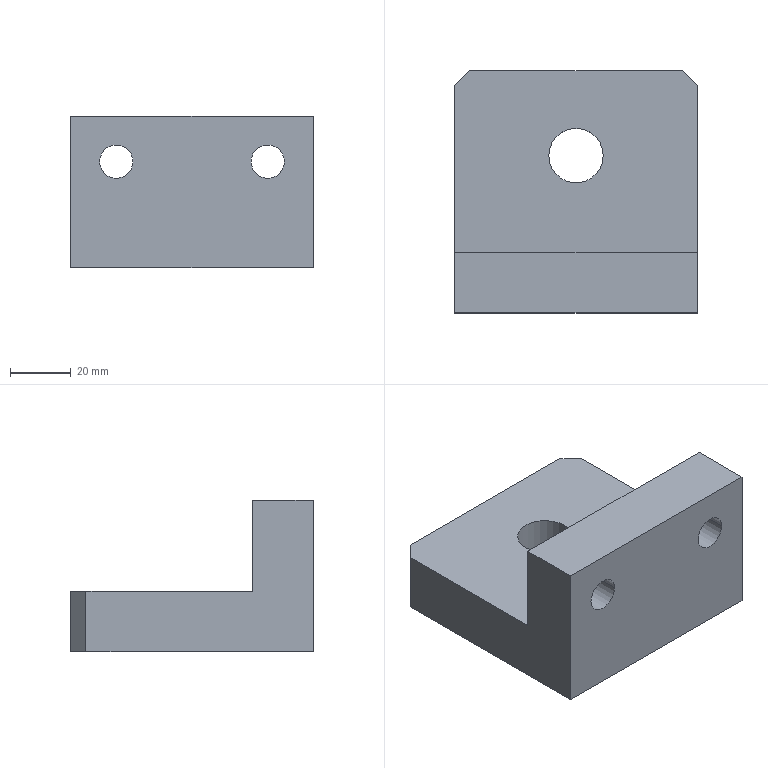Part | STEP file | DCV-000-032-B | 1 solid | 16 faces | box 80 x 80 x 50 mm | volume 166609 mm3 | plane 10 | cylinder 6 | commonest cylinder face diameters 11 x4 18 x2
STEP:
#1=CARTESIAN_POINT('',(0.,0.,0.));
#2=DIRECTION('',(0.,0.,1.));
#3=DIRECTION('',(1.,0.,0.));
#4=AXIS2_PLACEMENT_3D('',#1,#2,#3);
#5=CARTESIAN_POINT('',(30.5,0.,35.));
#6=VERTEX_POINT('',#5);
#7=CARTESIAN_POINT('',(30.5,20.,35.));
#8=VERTEX_POINT('',#7);
#9=CARTESIAN_POINT('',(30.5,-103.693,35.));
#10=DIRECTION('',(0.,1.,0.));
#11=VECTOR('',#10,1.);
#12=LINE('',#9,#11);
#13=CARTESIAN_POINT('',(25.,-103.693,35.));
#14=DIRECTION('',(0.,1.,0.));
#15=DIRECTION('',(1.,0.,0.));
#16=AXIS2_PLACEMENT_3D('',#13,#14,#15);
#17=CYLINDRICAL_SURFACE('',#16,5.5);
#18=CARTESIAN_POINT('',(6.283,0.));
#19=DIRECTION('',(0.,1.));
#20=VECTOR('',#19,1.);
#21=LINE('',#18,#20);
#22=(GEOMETRIC_REPRESENTATION_CONTEXT(2)PARAMETRIC_REPRESENTATION_CONTEXT()REPRESENTATION_CONTEXT('',''));
#23=DEFINITIONAL_REPRESENTATION('',(#21),#22);
#24=PCURVE('',#17,#23);
#25=CARTESIAN_POINT('',(25.,-103.693,35.));
#26=DIRECTION('',(0.,1.,0.));
#27=DIRECTION('',(1.,0.,0.));
#28=AXIS2_PLACEMENT_3D('',#25,#26,#27);
#29=CYLINDRICAL_SURFACE('',#28,5.5);
#30=CARTESIAN_POINT('',(0.,0.));
#31=DIRECTION('',(0.,1.));
#32=VECTOR('',#31,1.);
#33=LINE('',#30,#32);
#34=(GEOMETRIC_REPRESENTATION_CONTEXT(2)PARAMETRIC_REPRESENTATION_CONTEXT()REPRESENTATION_CONTEXT('',''));
#35=DEFINITIONAL_REPRESENTATION('',(#33),#34);
#36=PCURVE('',#29,#35);
#37=SURFACE_CURVE('',#12,(#24,#36),.PCURVE_S1.);
#38=EDGE_CURVE('',#6,#8,#37,.T.);
#39=ORIENTED_EDGE('',*,*,#38,.T.);
#40=CARTESIAN_POINT('',(19.5,20.,35.));
#41=VERTEX_POINT('',#40);
#42=CARTESIAN_POINT('',(25.,20.,35.));
#43=DIRECTION('',(0.,-1.,0.));
#44=DIRECTION('',(1.,0.,0.));
#45=AXIS2_PLACEMENT_3D('',#42,#43,#44);
#46=CIRCLE('',#45,5.5);
#47=CARTESIAN_POINT('',(6.283,123.693));
#48=DIRECTION('',(-1.,0.));
#49=VECTOR('',#48,1.);
#50=LINE('',#47,#49);
#51=(GEOMETRIC_REPRESENTATION_CONTEXT(2)PARAMETRIC_REPRESENTATION_CONTEXT()REPRESENTATION_CONTEXT('',''));
#52=DEFINITIONAL_REPRESENTATION('',(#50),#51);
#53=PCURVE('',#17,#52);
#54=CARTESIAN_POINT('',(40.,20.,20.));
#55=DIRECTION('',(0.,1.,0.));
#56=DIRECTION('',(1.,0.,0.));
#57=AXIS2_PLACEMENT_3D('',#54,#55,#56);
#58=PLANE('',#57);
#59=CARTESIAN_POINT('',(-9.5,-15.));
#60=CARTESIAN_POINT('',(-9.5,-24.526));
#61=CARTESIAN_POINT('',(-17.75,-19.763));
#62=CARTESIAN_POINT('',(-26.,-15.));
#63=CARTESIAN_POINT('',(-17.75,-10.237));
#64=CARTESIAN_POINT('',(-9.5,-5.474));
#65=CARTESIAN_POINT('',(-9.5,-15.));
#66=(BOUNDED_CURVE()B_SPLINE_CURVE(2,(#59,#60,#61,#62,#63,#64,#65),.UNSPECIFIED.,.T.,.F.)B_SPLINE_CURVE_WITH_KNOTS((1,2,2,2,2,1),(-2.094,0.,2.094,4.189,6.283,8.378),.UNSPECIFIED.)CURVE()GEOMETRIC_REPRESENTATION_ITEM()RATIONAL_B_SPLINE_CURVE((1.,0.5,1.,0.5,1.,0.5,1.))REPRESENTATION_ITEM(''));
#67=(GEOMETRIC_REPRESENTATION_CONTEXT(2)PARAMETRIC_REPRESENTATION_CONTEXT()REPRESENTATION_CONTEXT('',''));
#68=DEFINITIONAL_REPRESENTATION('',(#66),#67);
#69=PCURVE('',#58,#68);
#70=SURFACE_CURVE('',#46,(#53,#69),.PCURVE_S1.);
#71=EDGE_CURVE('',#8,#41,#70,.T.);
#72=ORIENTED_EDGE('',*,*,#71,.T.);
#73=CARTESIAN_POINT('',(19.5,0.,35.));
#74=VERTEX_POINT('',#73);
#75=CARTESIAN_POINT('',(19.5,-103.693,35.));
#76=DIRECTION('',(0.,1.,0.));
#77=VECTOR('',#76,1.);
#78=LINE('',#75,#77);
#79=CARTESIAN_POINT('',(3.142,0.));
#80=DIRECTION('',(0.,1.));
#81=VECTOR('',#80,1.);
#82=LINE('',#79,#81);
#83=(GEOMETRIC_REPRESENTATION_CONTEXT(2)PARAMETRIC_REPRESENTATION_CONTEXT()REPRESENTATION_CONTEXT('',''));
#84=DEFINITIONAL_REPRESENTATION('',(#82),#83);
#85=PCURVE('',#17,#84);
#86=CARTESIAN_POINT('',(3.142,0.));
#87=DIRECTION('',(0.,1.));
#88=VECTOR('',#87,1.);
#89=LINE('',#86,#88);
#90=(GEOMETRIC_REPRESENTATION_CONTEXT(2)PARAMETRIC_REPRESENTATION_CONTEXT()REPRESENTATION_CONTEXT('',''));
#91=DEFINITIONAL_REPRESENTATION('',(#89),#90);
#92=PCURVE('',#29,#91);
#93=SURFACE_CURVE('',#78,(#85,#92),.PCURVE_S1.);
#94=EDGE_CURVE('',#74,#41,#93,.T.);
#95=ORIENTED_EDGE('',*,*,#94,.F.);
#96=CARTESIAN_POINT('',(25.,0.,35.));
#97=DIRECTION('',(0.,1.,0.));
#98=DIRECTION('',(1.,0.,0.));
#99=AXIS2_PLACEMENT_3D('',#96,#97,#98);
#100=CIRCLE('',#99,5.5);
#101=CARTESIAN_POINT('',(0.,103.693));
#102=DIRECTION('',(1.,0.));
#103=VECTOR('',#102,1.);
#104=LINE('',#101,#103);
#105=(GEOMETRIC_REPRESENTATION_CONTEXT(2)PARAMETRIC_REPRESENTATION_CONTEXT()REPRESENTATION_CONTEXT('',''));
#106=DEFINITIONAL_REPRESENTATION('',(#104),#105);
#107=PCURVE('',#17,#106);
#108=CARTESIAN_POINT('',(-40.,0.,0.));
#109=DIRECTION('',(0.,-1.,0.));
#110=DIRECTION('',(0.,0.,-1.));
#111=AXIS2_PLACEMENT_3D('',#108,#109,#110);
#112=PLANE('',#111);
#113=CARTESIAN_POINT('',(-35.,70.5));
#114=CARTESIAN_POINT('',(-25.474,70.5));
#115=CARTESIAN_POINT('',(-30.237,62.25));
#116=CARTESIAN_POINT('',(-35.,54.));
#117=CARTESIAN_POINT('',(-39.763,62.25));
#118=CARTESIAN_POINT('',(-44.526,70.5));
#119=CARTESIAN_POINT('',(-35.,70.5));
#120=(BOUNDED_CURVE()B_SPLINE_CURVE(2,(#113,#114,#115,#116,#117,#118,#119),.UNSPECIFIED.,.T.,.F.)B_SPLINE_CURVE_WITH_KNOTS((1,2,2,2,2,1),(-2.094,0.,2.094,4.189,6.283,8.378),.UNSPECIFIED.)CURVE()GEOMETRIC_REPRESENTATION_ITEM()RATIONAL_B_SPLINE_CURVE((1.,0.5,1.,0.5,1.,0.5,1.))REPRESENTATION_ITEM(''));
#121=(GEOMETRIC_REPRESENTATION_CONTEXT(2)PARAMETRIC_REPRESENTATION_CONTEXT()REPRESENTATION_CONTEXT('',''));
#122=DEFINITIONAL_REPRESENTATION('',(#120),#121);
#123=PCURVE('',#112,#122);
#124=SURFACE_CURVE('',#100,(#107,#123),.PCURVE_S1.);
#125=EDGE_CURVE('',#74,#6,#124,.T.);
#126=ORIENTED_EDGE('',*,*,#125,.T.);
#127=EDGE_LOOP('',(#39,#72,#95,#126));
#128=FACE_BOUND('',#127,.F.);
#129=ADVANCED_FACE('',(#128),#17,.F.);
#130=CARTESIAN_POINT('',(-19.5,0.,35.));
#131=VERTEX_POINT('',#130);
#132=CARTESIAN_POINT('',(-19.5,20.,35.));
#133=VERTEX_POINT('',#132);
#134=CARTESIAN_POINT('',(-19.5,-103.693,35.));
#135=DIRECTION('',(0.,1.,0.));
#136=VECTOR('',#135,1.);
#137=LINE('',#134,#136);
#138=CARTESIAN_POINT('',(-25.,-103.693,35.));
#139=DIRECTION('',(0.,1.,0.));
#140=DIRECTION('',(1.,0.,0.));
#141=AXIS2_PLACEMENT_3D('',#138,#139,#140);
#142=CYLINDRICAL_SURFACE('',#141,5.5);
#143=CARTESIAN_POINT('',(6.283,0.));
#144=DIRECTION('',(0.,1.));
#145=VECTOR('',#144,1.);
#146=LINE('',#143,#145);
#147=(GEOMETRIC_REPRESENTATION_CONTEXT(2)PARAMETRIC_REPRESENTATION_CONTEXT()REPRESENTATION_CONTEXT('',''));
#148=DEFINITIONAL_REPRESENTATION('',(#146),#147);
#149=PCURVE('',#142,#148);
#150=CARTESIAN_POINT('',(-25.,-103.693,35.));
#151=DIRECTION('',(0.,1.,0.));
#152=DIRECTION('',(1.,0.,0.));
#153=AXIS2_PLACEMENT_3D('',#150,#151,#152);
#154=CYLINDRICAL_SURFACE('',#153,5.5);
#155=CARTESIAN_POINT('',(0.,0.));
#156=DIRECTION('',(0.,1.));
#157=VECTOR('',#156,1.);
#158=LINE('',#155,#157);
#159=(GEOMETRIC_REPRESENTATION_CONTEXT(2)PARAMETRIC_REPRESENTATION_CONTEXT()REPRESENTATION_CONTEXT('',''));
#160=DEFINITIONAL_REPRESENTATION('',(#158),#159);
#161=PCURVE('',#154,#160);
#162=SURFACE_CURVE('',#137,(#149,#161),.PCURVE_S1.);
#163=EDGE_CURVE('',#131,#133,#162,.T.);
#164=ORIENTED_EDGE('',*,*,#163,.T.);
#165=CARTESIAN_POINT('',(-30.5,20.,35.));
#166=VERTEX_POINT('',#165);
#167=CARTESIAN_POINT('',(-25.,20.,35.));
#168=DIRECTION('',(0.,-1.,0.));
#169=DIRECTION('',(1.,0.,0.));
#170=AXIS2_PLACEMENT_3D('',#167,#168,#169);
#171=CIRCLE('',#170,5.5);
#172=CARTESIAN_POINT('',(6.283,123.693));
#173=DIRECTION('',(-1.,0.));
#174=VECTOR('',#173,1.);
#175=LINE('',#172,#174);
#176=(GEOMETRIC_REPRESENTATION_CONTEXT(2)PARAMETRIC_REPRESENTATION_CONTEXT()REPRESENTATION_CONTEXT('',''));
#177=DEFINITIONAL_REPRESENTATION('',(#175),#176);
#178=PCURVE('',#142,#177);
#179=CARTESIAN_POINT('',(-59.5,-15.));
#180=CARTESIAN_POINT('',(-59.5,-24.526));
#181=CARTESIAN_POINT('',(-67.75,-19.763));
#182=CARTESIAN_POINT('',(-76.,-15.));
#183=CARTESIAN_POINT('',(-67.75,-10.237));
#184=CARTESIAN_POINT('',(-59.5,-5.474));
#185=CARTESIAN_POINT('',(-59.5,-15.));
#186=(BOUNDED_CURVE()B_SPLINE_CURVE(2,(#179,#180,#181,#182,#183,#184,#185),.UNSPECIFIED.,.T.,.F.)B_SPLINE_CURVE_WITH_KNOTS((1,2,2,2,2,1),(-2.094,0.,2.094,4.189,6.283,8.378),.UNSPECIFIED.)CURVE()GEOMETRIC_REPRESENTATION_ITEM()RATIONAL_B_SPLINE_CURVE((1.,0.5,1.,0.5,1.,0.5,1.))REPRESENTATION_ITEM(''));
#187=(GEOMETRIC_REPRESENTATION_CONTEXT(2)PARAMETRIC_REPRESENTATION_CONTEXT()REPRESENTATION_CONTEXT('',''));
#188=DEFINITIONAL_REPRESENTATION('',(#186),#187);
#189=PCURVE('',#58,#188);
#190=SURFACE_CURVE('',#171,(#178,#189),.PCURVE_S1.);
#191=EDGE_CURVE('',#133,#166,#190,.T.);
#192=ORIENTED_EDGE('',*,*,#191,.T.);
#193=CARTESIAN_POINT('',(-30.5,0.,35.));
#194=VERTEX_POINT('',#193);
#195=CARTESIAN_POINT('',(-30.5,-103.693,35.));
#196=DIRECTION('',(0.,1.,0.));
#197=VECTOR('',#196,1.);
#198=LINE('',#195,#197);
#199=CARTESIAN_POINT('',(3.142,0.));
#200=DIRECTION('',(0.,1.));
#201=VECTOR('',#200,1.);
#202=LINE('',#199,#201);
#203=(GEOMETRIC_REPRESENTATION_CONTEXT(2)PARAMETRIC_REPRESENTATION_CONTEXT()REPRESENTATION_CONTEXT('',''));
#204=DEFINITIONAL_REPRESENTATION('',(#202),#203);
#205=PCURVE('',#142,#204);
#206=CARTESIAN_POINT('',(3.142,0.));
#207=DIRECTION('',(0.,1.));
#208=VECTOR('',#207,1.);
#209=LINE('',#206,#208);
#210=(GEOMETRIC_REPRESENTATION_CONTEXT(2)PARAMETRIC_REPRESENTATION_CONTEXT()REPRESENTATION_CONTEXT('',''));
#211=DEFINITIONAL_REPRESENTATION('',(#209),#210);
#212=PCURVE('',#154,#211);
#213=SURFACE_CURVE('',#198,(#205,#212),.PCURVE_S1.);
#214=EDGE_CURVE('',#194,#166,#213,.T.);
#215=ORIENTED_EDGE('',*,*,#214,.F.);
#216=CARTESIAN_POINT('',(-25.,0.,35.));
#217=DIRECTION('',(0.,1.,0.));
#218=DIRECTION('',(1.,0.,0.));
#219=AXIS2_PLACEMENT_3D('',#216,#217,#218);
#220=CIRCLE('',#219,5.5);
#221=CARTESIAN_POINT('',(0.,103.693));
#222=DIRECTION('',(1.,0.));
#223=VECTOR('',#222,1.);
#224=LINE('',#221,#223);
#225=(GEOMETRIC_REPRESENTATION_CONTEXT(2)PARAMETRIC_REPRESENTATION_CONTEXT()REPRESENTATION_CONTEXT('',''));
#226=DEFINITIONAL_REPRESENTATION('',(#224),#225);
#227=PCURVE('',#142,#226);
#228=CARTESIAN_POINT('',(-35.,20.5));
#229=CARTESIAN_POINT('',(-25.474,20.5));
#230=CARTESIAN_POINT('',(-30.237,12.25));
#231=CARTESIAN_POINT('',(-35.,4.));
#232=CARTESIAN_POINT('',(-39.763,12.25));
#233=CARTESIAN_POINT('',(-44.526,20.5));
#234=CARTESIAN_POINT('',(-35.,20.5));
#235=(BOUNDED_CURVE()B_SPLINE_CURVE(2,(#228,#229,#230,#231,#232,#233,#234),.UNSPECIFIED.,.T.,.F.)B_SPLINE_CURVE_WITH_KNOTS((1,2,2,2,2,1),(-2.094,0.,2.094,4.189,6.283,8.378),.UNSPECIFIED.)CURVE()GEOMETRIC_REPRESENTATION_ITEM()RATIONAL_B_SPLINE_CURVE((1.,0.5,1.,0.5,1.,0.5,1.))REPRESENTATION_ITEM(''));
#236=(GEOMETRIC_REPRESENTATION_CONTEXT(2)PARAMETRIC_REPRESENTATION_CONTEXT()REPRESENTATION_CONTEXT('',''));
#237=DEFINITIONAL_REPRESENTATION('',(#235),#236);
#238=PCURVE('',#112,#237);
#239=SURFACE_CURVE('',#220,(#227,#238),.PCURVE_S1.);
#240=EDGE_CURVE('',#194,#131,#239,.T.);
#241=ORIENTED_EDGE('',*,*,#240,.T.);
#242=EDGE_LOOP('',(#164,#192,#215,#241));
#243=FACE_BOUND('',#242,.F.);
#244=ADVANCED_FACE('',(#243),#142,.F.);
#245=CARTESIAN_POINT('',(9.,52.,0.));
#246=VERTEX_POINT('',#245);
#247=CARTESIAN_POINT('',(9.,52.,20.));
#248=VERTEX_POINT('',#247);
#249=CARTESIAN_POINT('',(9.,52.,-94.891));
#250=DIRECTION('',(0.,0.,1.));
#251=VECTOR('',#250,1.);
#252=LINE('',#249,#251);
#253=CARTESIAN_POINT('',(0.,52.,-94.891));
#254=DIRECTION('',(0.,0.,1.));
#255=DIRECTION('',(1.,0.,0.));
#256=AXIS2_PLACEMENT_3D('',#253,#254,#255);
#257=CYLINDRICAL_SURFACE('',#256,9.);
#258=CARTESIAN_POINT('',(6.283,0.));
#259=DIRECTION('',(0.,1.));
#260=VECTOR('',#259,1.);
#261=LINE('',#258,#260);
#262=(GEOMETRIC_REPRESENTATION_CONTEXT(2)PARAMETRIC_REPRESENTATION_CONTEXT()REPRESENTATION_CONTEXT('',''));
#263=DEFINITIONAL_REPRESENTATION('',(#261),#262);
#264=PCURVE('',#257,#263);
#265=CARTESIAN_POINT('',(0.,52.,-94.891));
#266=DIRECTION('',(0.,0.,1.));
#267=DIRECTION('',(1.,0.,0.));
#268=AXIS2_PLACEMENT_3D('',#265,#266,#267);
#269=CYLINDRICAL_SURFACE('',#268,9.);
#270=CARTESIAN_POINT('',(0.,0.));
#271=DIRECTION('',(0.,1.));
#272=VECTOR('',#271,1.);
#273=LINE('',#270,#272);
#274=(GEOMETRIC_REPRESENTATION_CONTEXT(2)PARAMETRIC_REPRESENTATION_CONTEXT()REPRESENTATION_CONTEXT('',''));
#275=DEFINITIONAL_REPRESENTATION('',(#273),#274);
#276=PCURVE('',#269,#275);
#277=SURFACE_CURVE('',#252,(#264,#276),.PCURVE_S1.);
#278=EDGE_CURVE('',#246,#248,#277,.T.);
#279=ORIENTED_EDGE('',*,*,#278,.T.);
#280=CARTESIAN_POINT('',(-9.,52.,20.));
#281=VERTEX_POINT('',#280);
#282=CARTESIAN_POINT('',(0.,52.,20.));
#283=DIRECTION('',(0.,0.,-1.));
#284=DIRECTION('',(1.,0.,0.));
#285=AXIS2_PLACEMENT_3D('',#282,#283,#284);
#286=CIRCLE('',#285,9.);
#287=CARTESIAN_POINT('',(6.283,114.891));
#288=DIRECTION('',(-1.,0.));
#289=VECTOR('',#288,1.);
#290=LINE('',#287,#289);
#291=(GEOMETRIC_REPRESENTATION_CONTEXT(2)PARAMETRIC_REPRESENTATION_CONTEXT()REPRESENTATION_CONTEXT('',''));
#292=DEFINITIONAL_REPRESENTATION('',(#290),#291);
#293=PCURVE('',#257,#292);
#294=CARTESIAN_POINT('',(0.,40.,20.));
#295=DIRECTION('',(0.,0.,1.));
#296=DIRECTION('',(1.,0.,0.));
#297=AXIS2_PLACEMENT_3D('',#294,#295,#296);
#298=PLANE('',#297);
#299=CARTESIAN_POINT('',(9.,12.));
#300=CARTESIAN_POINT('',(9.,-3.588));
#301=CARTESIAN_POINT('',(-4.5,4.206));
#302=CARTESIAN_POINT('',(-18.,12.));
#303=CARTESIAN_POINT('',(-4.5,19.794));
#304=CARTESIAN_POINT('',(9.,27.588));
#305=CARTESIAN_POINT('',(9.,12.));
#306=(BOUNDED_CURVE()B_SPLINE_CURVE(2,(#299,#300,#301,#302,#303,#304,#305),.UNSPECIFIED.,.T.,.F.)B_SPLINE_CURVE_WITH_KNOTS((1,2,2,2,2,1),(-2.094,0.,2.094,4.189,6.283,8.378),.UNSPECIFIED.)CURVE()GEOMETRIC_REPRESENTATION_ITEM()RATIONAL_B_SPLINE_CURVE((1.,0.5,1.,0.5,1.,0.5,1.))REPRESENTATION_ITEM(''));
#307=(GEOMETRIC_REPRESENTATION_CONTEXT(2)PARAMETRIC_REPRESENTATION_CONTEXT()REPRESENTATION_CONTEXT('',''));
#308=DEFINITIONAL_REPRESENTATION('',(#306),#307);
#309=PCURVE('',#298,#308);
#310=SURFACE_CURVE('',#286,(#293,#309),.PCURVE_S1.);
#311=EDGE_CURVE('',#248,#281,#310,.T.);
#312=ORIENTED_EDGE('',*,*,#311,.T.);
#313=CARTESIAN_POINT('',(-9.,52.,0.));
#314=VERTEX_POINT('',#313);
#315=CARTESIAN_POINT('',(-9.,52.,-94.891));
#316=DIRECTION('',(0.,0.,1.));
#317=VECTOR('',#316,1.);
#318=LINE('',#315,#317);
#319=CARTESIAN_POINT('',(3.142,0.));
#320=DIRECTION('',(0.,1.));
#321=VECTOR('',#320,1.);
#322=LINE('',#319,#321);
#323=(GEOMETRIC_REPRESENTATION_CONTEXT(2)PARAMETRIC_REPRESENTATION_CONTEXT()REPRESENTATION_CONTEXT('',''));
#324=DEFINITIONAL_REPRESENTATION('',(#322),#323);
#325=PCURVE('',#257,#324);
#326=CARTESIAN_POINT('',(3.142,0.));
#327=DIRECTION('',(0.,1.));
#328=VECTOR('',#327,1.);
#329=LINE('',#326,#328);
#330=(GEOMETRIC_REPRESENTATION_CONTEXT(2)PARAMETRIC_REPRESENTATION_CONTEXT()REPRESENTATION_CONTEXT('',''));
#331=DEFINITIONAL_REPRESENTATION('',(#329),#330);
#332=PCURVE('',#269,#331);
#333=SURFACE_CURVE('',#318,(#325,#332),.PCURVE_S1.);
#334=EDGE_CURVE('',#314,#281,#333,.T.);
#335=ORIENTED_EDGE('',*,*,#334,.F.);
#336=CARTESIAN_POINT('',(0.,52.,0.));
#337=DIRECTION('',(0.,0.,1.));
#338=DIRECTION('',(1.,0.,0.));
#339=AXIS2_PLACEMENT_3D('',#336,#337,#338);
#340=CIRCLE('',#339,9.);
#341=CARTESIAN_POINT('',(0.,94.891));
#342=DIRECTION('',(1.,0.));
#343=VECTOR('',#342,1.);
#344=LINE('',#341,#343);
#345=(GEOMETRIC_REPRESENTATION_CONTEXT(2)PARAMETRIC_REPRESENTATION_CONTEXT()REPRESENTATION_CONTEXT('',''));
#346=DEFINITIONAL_REPRESENTATION('',(#344),#345);
#347=PCURVE('',#257,#346);
#348=CARTESIAN_POINT('',(0.,40.,0.));
#349=DIRECTION('',(0.,0.,1.));
#350=DIRECTION('',(1.,0.,0.));
#351=AXIS2_PLACEMENT_3D('',#348,#349,#350);
#352=PLANE('',#351);
#353=CARTESIAN_POINT('',(0.,12.));
#354=DIRECTION('',(1.,0.));
#355=AXIS2_PLACEMENT_2D('',#353,#354);
#356=CIRCLE('',#355,9.);
#357=(GEOMETRIC_REPRESENTATION_CONTEXT(2)PARAMETRIC_REPRESENTATION_CONTEXT()REPRESENTATION_CONTEXT('',''));
#358=DEFINITIONAL_REPRESENTATION('',(#356),#357);
#359=PCURVE('',#352,#358);
#360=SURFACE_CURVE('',#340,(#347,#359),.PCURVE_S1.);
#361=EDGE_CURVE('',#314,#246,#360,.T.);
#362=ORIENTED_EDGE('',*,*,#361,.T.);
#363=EDGE_LOOP('',(#279,#312,#335,#362));
#364=FACE_BOUND('',#363,.F.);
#365=ADVANCED_FACE('',(#364),#257,.F.);
#366=ORIENTED_EDGE('',*,*,#311,.T.);
#367=CARTESIAN_POINT('',(0.,52.,20.));
#368=DIRECTION('',(0.,0.,-1.));
#369=DIRECTION('',(1.,0.,0.));
#370=AXIS2_PLACEMENT_3D('',#367,#368,#369);
#371=CIRCLE('',#370,9.);
#372=CARTESIAN_POINT('',(9.,12.));
#373=CARTESIAN_POINT('',(9.,-3.588));
#374=CARTESIAN_POINT('',(-4.5,4.206));
#375=CARTESIAN_POINT('',(-18.,12.));
#376=CARTESIAN_POINT('',(-4.5,19.794));
#377=CARTESIAN_POINT('',(9.,27.588));
#378=CARTESIAN_POINT('',(9.,12.));
#379=(BOUNDED_CURVE()B_SPLINE_CURVE(2,(#372,#373,#374,#375,#376,#377,#378),.UNSPECIFIED.,.T.,.F.)B_SPLINE_CURVE_WITH_KNOTS((1,2,2,2,2,1),(-2.094,0.,2.094,4.189,6.283,8.378),.UNSPECIFIED.)CURVE()GEOMETRIC_REPRESENTATION_ITEM()RATIONAL_B_SPLINE_CURVE((1.,0.5,1.,0.5,1.,0.5,1.))REPRESENTATION_ITEM(''));
#380=(GEOMETRIC_REPRESENTATION_CONTEXT(2)PARAMETRIC_REPRESENTATION_CONTEXT()REPRESENTATION_CONTEXT('',''));
#381=DEFINITIONAL_REPRESENTATION('',(#379),#380);
#382=PCURVE('',#298,#381);
#383=CARTESIAN_POINT('',(6.283,114.891));
#384=DIRECTION('',(-1.,0.));
#385=VECTOR('',#384,1.);
#386=LINE('',#383,#385);
#387=(GEOMETRIC_REPRESENTATION_CONTEXT(2)PARAMETRIC_REPRESENTATION_CONTEXT()REPRESENTATION_CONTEXT('',''));
#388=DEFINITIONAL_REPRESENTATION('',(#386),#387);
#389=PCURVE('',#269,#388);
#390=SURFACE_CURVE('',#371,(#382,#389),.PCURVE_S1.);
#391=EDGE_CURVE('',#281,#248,#390,.T.);
#392=ORIENTED_EDGE('',*,*,#391,.T.);
#393=EDGE_LOOP('',(#366,#392));
#394=FACE_BOUND('',#393,.T.);
#395=CARTESIAN_POINT('',(-40.,75.,20.));
#396=VERTEX_POINT('',#395);
#397=CARTESIAN_POINT('',(-35.,80.,20.));
#398=VERTEX_POINT('',#397);
#399=CARTESIAN_POINT('',(-37.5,77.5,20.));
#400=DIRECTION('',(0.7071,0.7071,0.));
#401=VECTOR('',#400,1.);
#402=LINE('',#399,#401);
#403=CARTESIAN_POINT('',(-37.5,37.5));
#404=DIRECTION('',(0.7071,0.7071));
#405=VECTOR('',#404,1.);
#406=LINE('',#403,#405);
#407=(GEOMETRIC_REPRESENTATION_CONTEXT(2)PARAMETRIC_REPRESENTATION_CONTEXT()REPRESENTATION_CONTEXT('',''));
#408=DEFINITIONAL_REPRESENTATION('',(#406),#407);
#409=PCURVE('',#298,#408);
#410=CARTESIAN_POINT('',(-37.5,77.5,0.));
#411=DIRECTION('',(-0.7071,0.7071,0.));
#412=DIRECTION('',(0.,0.,1.));
#413=AXIS2_PLACEMENT_3D('',#410,#411,#412);
#414=PLANE('',#413);
#415=CARTESIAN_POINT('',(20.,0.));
#416=DIRECTION('',(0.,1.));
#417=VECTOR('',#416,1.);
#418=LINE('',#415,#417);
#419=(GEOMETRIC_REPRESENTATION_CONTEXT(2)PARAMETRIC_REPRESENTATION_CONTEXT()REPRESENTATION_CONTEXT('',''));
#420=DEFINITIONAL_REPRESENTATION('',(#418),#419);
#421=PCURVE('',#414,#420);
#422=SURFACE_CURVE('',#402,(#409,#421),.PCURVE_S1.);
#423=EDGE_CURVE('',#396,#398,#422,.T.);
#424=ORIENTED_EDGE('',*,*,#423,.F.);
#425=CARTESIAN_POINT('',(-40.,20.,20.));
#426=VERTEX_POINT('',#425);
#427=CARTESIAN_POINT('',(-40.,80.,20.));
#428=DIRECTION('',(0.,-1.,0.));
#429=VECTOR('',#428,1.);
#430=LINE('',#427,#429);
#431=CARTESIAN_POINT('',(-40.,40.));
#432=DIRECTION('',(0.,-1.));
#433=VECTOR('',#432,1.);
#434=LINE('',#431,#433);
#435=(GEOMETRIC_REPRESENTATION_CONTEXT(2)PARAMETRIC_REPRESENTATION_CONTEXT()REPRESENTATION_CONTEXT('',''));
#436=DEFINITIONAL_REPRESENTATION('',(#434),#435);
#437=PCURVE('',#298,#436);
#438=CARTESIAN_POINT('',(-40.,80.,0.));
#439=DIRECTION('',(-1.,0.,0.));
#440=DIRECTION('',(0.,1.,0.));
#441=AXIS2_PLACEMENT_3D('',#438,#439,#440);
#442=PLANE('',#441);
#443=CARTESIAN_POINT('',(0.,-20.));
#444=DIRECTION('',(-1.,0.));
#445=VECTOR('',#444,1.);
#446=LINE('',#443,#445);
#447=(GEOMETRIC_REPRESENTATION_CONTEXT(2)PARAMETRIC_REPRESENTATION_CONTEXT()REPRESENTATION_CONTEXT('',''));
#448=DEFINITIONAL_REPRESENTATION('',(#446),#447);
#449=PCURVE('',#442,#448);
#450=SURFACE_CURVE('',#430,(#437,#449),.PCURVE_S1.);
#451=EDGE_CURVE('',#396,#426,#450,.T.);
#452=ORIENTED_EDGE('',*,*,#451,.T.);
#453=CARTESIAN_POINT('',(40.,20.,20.));
#454=VERTEX_POINT('',#453);
#455=CARTESIAN_POINT('',(20.,20.,20.));
#456=DIRECTION('',(1.,0.,0.));
#457=VECTOR('',#456,1.);
#458=LINE('',#455,#457);
#459=CARTESIAN_POINT('',(20.,-20.));
#460=DIRECTION('',(1.,0.));
#461=VECTOR('',#460,1.);
#462=LINE('',#459,#461);
#463=(GEOMETRIC_REPRESENTATION_CONTEXT(2)PARAMETRIC_REPRESENTATION_CONTEXT()REPRESENTATION_CONTEXT('',''));
#464=DEFINITIONAL_REPRESENTATION('',(#462),#463);
#465=PCURVE('',#298,#464);
#466=CARTESIAN_POINT('',(-20.,0.));
#467=DIRECTION('',(1.,0.));
#468=VECTOR('',#467,1.);
#469=LINE('',#466,#468);
#470=(GEOMETRIC_REPRESENTATION_CONTEXT(2)PARAMETRIC_REPRESENTATION_CONTEXT()REPRESENTATION_CONTEXT('',''));
#471=DEFINITIONAL_REPRESENTATION('',(#469),#470);
#472=PCURVE('',#58,#471);
#473=SURFACE_CURVE('',#458,(#465,#472),.PCURVE_S1.);
#474=EDGE_CURVE('',#426,#454,#473,.T.);
#475=ORIENTED_EDGE('',*,*,#474,.T.);
#476=CARTESIAN_POINT('',(40.,75.,20.));
#477=VERTEX_POINT('',#476);
#478=CARTESIAN_POINT('',(40.,0.,20.));
#479=DIRECTION('',(0.,1.,0.));
#480=VECTOR('',#479,1.);
#481=LINE('',#478,#480);
#482=CARTESIAN_POINT('',(40.,-40.));
#483=DIRECTION('',(0.,1.));
#484=VECTOR('',#483,1.);
#485=LINE('',#482,#484);
#486=(GEOMETRIC_REPRESENTATION_CONTEXT(2)PARAMETRIC_REPRESENTATION_CONTEXT()REPRESENTATION_CONTEXT('',''));
#487=DEFINITIONAL_REPRESENTATION('',(#485),#486);
#488=PCURVE('',#298,#487);
#489=CARTESIAN_POINT('',(40.,0.,0.));
#490=DIRECTION('',(1.,0.,0.));
#491=DIRECTION('',(0.,-1.,0.));
#492=AXIS2_PLACEMENT_3D('',#489,#490,#491);
#493=PLANE('',#492);
#494=CARTESIAN_POINT('',(0.,-20.));
#495=DIRECTION('',(-1.,0.));
#496=VECTOR('',#495,1.);
#497=LINE('',#494,#496);
#498=(GEOMETRIC_REPRESENTATION_CONTEXT(2)PARAMETRIC_REPRESENTATION_CONTEXT()REPRESENTATION_CONTEXT('',''));
#499=DEFINITIONAL_REPRESENTATION('',(#497),#498);
#500=PCURVE('',#493,#499);
#501=SURFACE_CURVE('',#481,(#488,#500),.PCURVE_S1.);
#502=EDGE_CURVE('',#454,#477,#501,.T.);
#503=ORIENTED_EDGE('',*,*,#502,.T.);
#504=CARTESIAN_POINT('',(35.,80.,20.));
#505=VERTEX_POINT('',#504);
#506=CARTESIAN_POINT('',(37.5,77.5,20.));
#507=DIRECTION('',(0.7071,-0.7071,0.));
#508=VECTOR('',#507,1.);
#509=LINE('',#506,#508);
#510=CARTESIAN_POINT('',(37.5,37.5));
#511=DIRECTION('',(0.7071,-0.7071));
#512=VECTOR('',#511,1.);
#513=LINE('',#510,#512);
#514=(GEOMETRIC_REPRESENTATION_CONTEXT(2)PARAMETRIC_REPRESENTATION_CONTEXT()REPRESENTATION_CONTEXT('',''));
#515=DEFINITIONAL_REPRESENTATION('',(#513),#514);
#516=PCURVE('',#298,#515);
#517=CARTESIAN_POINT('',(37.5,77.5,0.));
#518=DIRECTION('',(0.7071,0.7071,0.));
#519=DIRECTION('',(0.,0.,-1.));
#520=AXIS2_PLACEMENT_3D('',#517,#518,#519);
#521=PLANE('',#520);
#522=CARTESIAN_POINT('',(-20.,0.));
#523=DIRECTION('',(0.,-1.));
#524=VECTOR('',#523,1.);
#525=LINE('',#522,#524);
#526=(GEOMETRIC_REPRESENTATION_CONTEXT(2)PARAMETRIC_REPRESENTATION_CONTEXT()REPRESENTATION_CONTEXT('',''));
#527=DEFINITIONAL_REPRESENTATION('',(#525),#526);
#528=PCURVE('',#521,#527);
#529=SURFACE_CURVE('',#509,(#516,#528),.PCURVE_S1.);
#530=EDGE_CURVE('',#505,#477,#529,.T.);
#531=ORIENTED_EDGE('',*,*,#530,.F.);
#532=CARTESIAN_POINT('',(40.,80.,20.));
#533=DIRECTION('',(-1.,0.,0.));
#534=VECTOR('',#533,1.);
#535=LINE('',#532,#534);
#536=CARTESIAN_POINT('',(40.,40.));
#537=DIRECTION('',(-1.,0.));
#538=VECTOR('',#537,1.);
#539=LINE('',#536,#538);
#540=(GEOMETRIC_REPRESENTATION_CONTEXT(2)PARAMETRIC_REPRESENTATION_CONTEXT()REPRESENTATION_CONTEXT('',''));
#541=DEFINITIONAL_REPRESENTATION('',(#539),#540);
#542=PCURVE('',#298,#541);
#543=CARTESIAN_POINT('',(40.,80.,0.));
#544=DIRECTION('',(0.,1.,0.));
#545=DIRECTION('',(1.,0.,0.));
#546=AXIS2_PLACEMENT_3D('',#543,#544,#545);
#547=PLANE('',#546);
#548=CARTESIAN_POINT('',(0.,-20.));
#549=DIRECTION('',(-1.,0.));
#550=VECTOR('',#549,1.);
#551=LINE('',#548,#550);
#552=(GEOMETRIC_REPRESENTATION_CONTEXT(2)PARAMETRIC_REPRESENTATION_CONTEXT()REPRESENTATION_CONTEXT('',''));
#553=DEFINITIONAL_REPRESENTATION('',(#551),#552);
#554=PCURVE('',#547,#553);
#555=SURFACE_CURVE('',#535,(#542,#554),.PCURVE_S1.);
#556=EDGE_CURVE('',#505,#398,#555,.T.);
#557=ORIENTED_EDGE('',*,*,#556,.T.);
#558=EDGE_LOOP('',(#424,#452,#475,#503,#531,#557));
#559=FACE_BOUND('',#558,.T.);
#560=ADVANCED_FACE('',(#394,#559),#298,.T.);
#561=CARTESIAN_POINT('',(-35.,80.,0.));
#562=VERTEX_POINT('',#561);
#563=CARTESIAN_POINT('',(-35.,80.,0.));
#564=DIRECTION('',(0.,0.,-1.));
#565=VECTOR('',#564,1.);
#566=LINE('',#563,#565);
#567=CARTESIAN_POINT('',(-75.,0.));
#568=DIRECTION('',(0.,1.));
#569=VECTOR('',#568,1.);
#570=LINE('',#567,#569);
#571=(GEOMETRIC_REPRESENTATION_CONTEXT(2)PARAMETRIC_REPRESENTATION_CONTEXT()REPRESENTATION_CONTEXT('',''));
#572=DEFINITIONAL_REPRESENTATION('',(#570),#571);
#573=PCURVE('',#547,#572);
#574=CARTESIAN_POINT('',(0.,3.536));
#575=DIRECTION('',(-1.,0.));
#576=VECTOR('',#575,1.);
#577=LINE('',#574,#576);
#578=(GEOMETRIC_REPRESENTATION_CONTEXT(2)PARAMETRIC_REPRESENTATION_CONTEXT()REPRESENTATION_CONTEXT('',''));
#579=DEFINITIONAL_REPRESENTATION('',(#577),#578);
#580=PCURVE('',#414,#579);
#581=SURFACE_CURVE('',#566,(#573,#580),.PCURVE_S1.);
#582=EDGE_CURVE('',#398,#562,#581,.T.);
#583=ORIENTED_EDGE('',*,*,#582,.F.);
#584=ORIENTED_EDGE('',*,*,#556,.F.);
#585=CARTESIAN_POINT('',(35.,80.,0.));
#586=VERTEX_POINT('',#585);
#587=CARTESIAN_POINT('',(35.,80.,0.));
#588=DIRECTION('',(0.,0.,1.));
#589=VECTOR('',#588,1.);
#590=LINE('',#587,#589);
#591=CARTESIAN_POINT('',(-5.,0.));
#592=DIRECTION('',(0.,-1.));
#593=VECTOR('',#592,1.);
#594=LINE('',#591,#593);
#595=(GEOMETRIC_REPRESENTATION_CONTEXT(2)PARAMETRIC_REPRESENTATION_CONTEXT()REPRESENTATION_CONTEXT('',''));
#596=DEFINITIONAL_REPRESENTATION('',(#594),#595);
#597=PCURVE('',#547,#596);
#598=CARTESIAN_POINT('',(0.,3.536));
#599=DIRECTION('',(-1.,0.));
#600=VECTOR('',#599,1.);
#601=LINE('',#598,#600);
#602=(GEOMETRIC_REPRESENTATION_CONTEXT(2)PARAMETRIC_REPRESENTATION_CONTEXT()REPRESENTATION_CONTEXT('',''));
#603=DEFINITIONAL_REPRESENTATION('',(#601),#602);
#604=PCURVE('',#521,#603);
#605=SURFACE_CURVE('',#590,(#597,#604),.PCURVE_S1.);
#606=EDGE_CURVE('',#586,#505,#605,.T.);
#607=ORIENTED_EDGE('',*,*,#606,.F.);
#608=CARTESIAN_POINT('',(40.,80.,0.));
#609=DIRECTION('',(-1.,0.,0.));
#610=VECTOR('',#609,1.);
#611=LINE('',#608,#610);
#612=CARTESIAN_POINT('',(0.,0.));
#613=DIRECTION('',(-1.,0.));
#614=VECTOR('',#613,1.);
#615=LINE('',#612,#614);
#616=(GEOMETRIC_REPRESENTATION_CONTEXT(2)PARAMETRIC_REPRESENTATION_CONTEXT()REPRESENTATION_CONTEXT('',''));
#617=DEFINITIONAL_REPRESENTATION('',(#615),#616);
#618=PCURVE('',#547,#617);
#619=CARTESIAN_POINT('',(40.,40.));
#620=DIRECTION('',(-1.,0.));
#621=VECTOR('',#620,1.);
#622=LINE('',#619,#621);
#623=(GEOMETRIC_REPRESENTATION_CONTEXT(2)PARAMETRIC_REPRESENTATION_CONTEXT()REPRESENTATION_CONTEXT('',''));
#624=DEFINITIONAL_REPRESENTATION('',(#622),#623);
#625=PCURVE('',#352,#624);
#626=SURFACE_CURVE('',#611,(#618,#625),.PCURVE_S1.);
#627=EDGE_CURVE('',#586,#562,#626,.T.);
#628=ORIENTED_EDGE('',*,*,#627,.T.);
#629=EDGE_LOOP('',(#583,#584,#607,#628));
#630=FACE_BOUND('',#629,.T.);
#631=ADVANCED_FACE('',(#630),#547,.T.);
#632=CARTESIAN_POINT('',(-25.,0.,35.));
#633=DIRECTION('',(0.,1.,0.));
#634=DIRECTION('',(1.,0.,0.));
#635=AXIS2_PLACEMENT_3D('',#632,#633,#634);
#636=CIRCLE('',#635,5.5);
#637=CARTESIAN_POINT('',(-35.,20.5));
#638=CARTESIAN_POINT('',(-25.474,20.5));
#639=CARTESIAN_POINT('',(-30.237,12.25));
#640=CARTESIAN_POINT('',(-35.,4.));
#641=CARTESIAN_POINT('',(-39.763,12.25));
#642=CARTESIAN_POINT('',(-44.526,20.5));
#643=CARTESIAN_POINT('',(-35.,20.5));
#644=(BOUNDED_CURVE()B_SPLINE_CURVE(2,(#637,#638,#639,#640,#641,#642,#643),.UNSPECIFIED.,.T.,.F.)B_SPLINE_CURVE_WITH_KNOTS((1,2,2,2,2,1),(-2.094,0.,2.094,4.189,6.283,8.378),.UNSPECIFIED.)CURVE()GEOMETRIC_REPRESENTATION_ITEM()RATIONAL_B_SPLINE_CURVE((1.,0.5,1.,0.5,1.,0.5,1.))REPRESENTATION_ITEM(''));
#645=(GEOMETRIC_REPRESENTATION_CONTEXT(2)PARAMETRIC_REPRESENTATION_CONTEXT()REPRESENTATION_CONTEXT('',''));
#646=DEFINITIONAL_REPRESENTATION('',(#644),#645);
#647=PCURVE('',#112,#646);
#648=CARTESIAN_POINT('',(0.,103.693));
#649=DIRECTION('',(1.,0.));
#650=VECTOR('',#649,1.);
#651=LINE('',#648,#650);
#652=(GEOMETRIC_REPRESENTATION_CONTEXT(2)PARAMETRIC_REPRESENTATION_CONTEXT()REPRESENTATION_CONTEXT('',''));
#653=DEFINITIONAL_REPRESENTATION('',(#651),#652);
#654=PCURVE('',#154,#653);
#655=SURFACE_CURVE('',#636,(#647,#654),.PCURVE_S1.);
#656=EDGE_CURVE('',#131,#194,#655,.T.);
#657=ORIENTED_EDGE('',*,*,#656,.T.);
#658=ORIENTED_EDGE('',*,*,#240,.T.);
#659=EDGE_LOOP('',(#657,#658));
#660=FACE_BOUND('',#659,.T.);
#661=CARTESIAN_POINT('',(25.,0.,35.));
#662=DIRECTION('',(0.,1.,0.));
#663=DIRECTION('',(1.,0.,0.));
#664=AXIS2_PLACEMENT_3D('',#661,#662,#663);
#665=CIRCLE('',#664,5.5);
#666=CARTESIAN_POINT('',(-35.,70.5));
#667=CARTESIAN_POINT('',(-25.474,70.5));
#668=CARTESIAN_POINT('',(-30.237,62.25));
#669=CARTESIAN_POINT('',(-35.,54.));
#670=CARTESIAN_POINT('',(-39.763,62.25));
#671=CARTESIAN_POINT('',(-44.526,70.5));
#672=CARTESIAN_POINT('',(-35.,70.5));
#673=(BOUNDED_CURVE()B_SPLINE_CURVE(2,(#666,#667,#668,#669,#670,#671,#672),.UNSPECIFIED.,.T.,.F.)B_SPLINE_CURVE_WITH_KNOTS((1,2,2,2,2,1),(-2.094,0.,2.094,4.189,6.283,8.378),.UNSPECIFIED.)CURVE()GEOMETRIC_REPRESENTATION_ITEM()RATIONAL_B_SPLINE_CURVE((1.,0.5,1.,0.5,1.,0.5,1.))REPRESENTATION_ITEM(''));
#674=(GEOMETRIC_REPRESENTATION_CONTEXT(2)PARAMETRIC_REPRESENTATION_CONTEXT()REPRESENTATION_CONTEXT('',''));
#675=DEFINITIONAL_REPRESENTATION('',(#673),#674);
#676=PCURVE('',#112,#675);
#677=CARTESIAN_POINT('',(0.,103.693));
#678=DIRECTION('',(1.,0.));
#679=VECTOR('',#678,1.);
#680=LINE('',#677,#679);
#681=(GEOMETRIC_REPRESENTATION_CONTEXT(2)PARAMETRIC_REPRESENTATION_CONTEXT()REPRESENTATION_CONTEXT('',''));
#682=DEFINITIONAL_REPRESENTATION('',(#680),#681);
#683=PCURVE('',#29,#682);
#684=SURFACE_CURVE('',#665,(#676,#683),.PCURVE_S1.);
#685=EDGE_CURVE('',#6,#74,#684,.T.);
#686=ORIENTED_EDGE('',*,*,#685,.T.);
#687=ORIENTED_EDGE('',*,*,#125,.T.);
#688=EDGE_LOOP('',(#686,#687));
#689=FACE_BOUND('',#688,.T.);
#690=CARTESIAN_POINT('',(-40.,0.,0.));
#691=VERTEX_POINT('',#690);
#692=CARTESIAN_POINT('',(40.,0.,0.));
#693=VERTEX_POINT('',#692);
#694=CARTESIAN_POINT('',(-40.,0.,0.));
#695=DIRECTION('',(1.,0.,0.));
#696=VECTOR('',#695,1.);
#697=LINE('',#694,#696);
#698=CARTESIAN_POINT('',(0.,0.));
#699=DIRECTION('',(0.,1.));
#700=VECTOR('',#699,1.);
#701=LINE('',#698,#700);
#702=(GEOMETRIC_REPRESENTATION_CONTEXT(2)PARAMETRIC_REPRESENTATION_CONTEXT()REPRESENTATION_CONTEXT('',''));
#703=DEFINITIONAL_REPRESENTATION('',(#701),#702);
#704=PCURVE('',#112,#703);
#705=CARTESIAN_POINT('',(-40.,-40.));
#706=DIRECTION('',(1.,0.));
#707=VECTOR('',#706,1.);
#708=LINE('',#705,#707);
#709=(GEOMETRIC_REPRESENTATION_CONTEXT(2)PARAMETRIC_REPRESENTATION_CONTEXT()REPRESENTATION_CONTEXT('',''));
#710=DEFINITIONAL_REPRESENTATION('',(#708),#709);
#711=PCURVE('',#352,#710);
#712=SURFACE_CURVE('',#697,(#704,#711),.PCURVE_S1.);
#713=EDGE_CURVE('',#691,#693,#712,.T.);
#714=ORIENTED_EDGE('',*,*,#713,.T.);
#715=CARTESIAN_POINT('',(40.,0.,50.));
#716=VERTEX_POINT('',#715);
#717=CARTESIAN_POINT('',(40.,0.,0.));
#718=DIRECTION('',(0.,0.,1.));
#719=VECTOR('',#718,1.);
#720=LINE('',#717,#719);
#721=CARTESIAN_POINT('',(0.,80.));
#722=DIRECTION('',(-1.,0.));
#723=VECTOR('',#722,1.);
#724=LINE('',#721,#723);
#725=(GEOMETRIC_REPRESENTATION_CONTEXT(2)PARAMETRIC_REPRESENTATION_CONTEXT()REPRESENTATION_CONTEXT('',''));
#726=DEFINITIONAL_REPRESENTATION('',(#724),#725);
#727=PCURVE('',#112,#726);
#728=CARTESIAN_POINT('',(0.,0.));
#729=DIRECTION('',(0.,-1.));
#730=VECTOR('',#729,1.);
#731=LINE('',#728,#730);
#732=(GEOMETRIC_REPRESENTATION_CONTEXT(2)PARAMETRIC_REPRESENTATION_CONTEXT()REPRESENTATION_CONTEXT('',''));
#733=DEFINITIONAL_REPRESENTATION('',(#731),#732);
#734=PCURVE('',#493,#733);
#735=SURFACE_CURVE('',#720,(#727,#734),.PCURVE_S1.);
#736=EDGE_CURVE('',#693,#716,#735,.T.);
#737=ORIENTED_EDGE('',*,*,#736,.T.);
#738=CARTESIAN_POINT('',(-40.,0.,50.));
#739=VERTEX_POINT('',#738);
#740=CARTESIAN_POINT('',(-40.,0.,50.));
#741=DIRECTION('',(1.,0.,0.));
#742=VECTOR('',#741,1.);
#743=LINE('',#740,#742);
#744=CARTESIAN_POINT('',(-50.,0.));
#745=DIRECTION('',(0.,1.));
#746=VECTOR('',#745,1.);
#747=LINE('',#744,#746);
#748=(GEOMETRIC_REPRESENTATION_CONTEXT(2)PARAMETRIC_REPRESENTATION_CONTEXT()REPRESENTATION_CONTEXT('',''));
#749=DEFINITIONAL_REPRESENTATION('',(#747),#748);
#750=PCURVE('',#112,#749);
#751=CARTESIAN_POINT('',(0.,10.,50.));
#752=DIRECTION('',(0.,0.,1.));
#753=DIRECTION('',(1.,0.,0.));
#754=AXIS2_PLACEMENT_3D('',#751,#752,#753);
#755=PLANE('',#754);
#756=CARTESIAN_POINT('',(-40.,-10.));
#757=DIRECTION('',(1.,0.));
#758=VECTOR('',#757,1.);
#759=LINE('',#756,#758);
#760=(GEOMETRIC_REPRESENTATION_CONTEXT(2)PARAMETRIC_REPRESENTATION_CONTEXT()REPRESENTATION_CONTEXT('',''));
#761=DEFINITIONAL_REPRESENTATION('',(#759),#760);
#762=PCURVE('',#755,#761);
#763=SURFACE_CURVE('',#743,(#750,#762),.PCURVE_S1.);
#764=EDGE_CURVE('',#739,#716,#763,.T.);
#765=ORIENTED_EDGE('',*,*,#764,.F.);
#766=CARTESIAN_POINT('',(-40.,0.,0.));
#767=DIRECTION('',(0.,0.,1.));
#768=VECTOR('',#767,1.);
#769=LINE('',#766,#768);
#770=CARTESIAN_POINT('',(0.,0.));
#771=DIRECTION('',(-1.,0.));
#772=VECTOR('',#771,1.);
#773=LINE('',#770,#772);
#774=(GEOMETRIC_REPRESENTATION_CONTEXT(2)PARAMETRIC_REPRESENTATION_CONTEXT()REPRESENTATION_CONTEXT('',''));
#775=DEFINITIONAL_REPRESENTATION('',(#773),#774);
#776=PCURVE('',#112,#775);
#777=CARTESIAN_POINT('',(-80.,0.));
#778=DIRECTION('',(0.,-1.));
#779=VECTOR('',#778,1.);
#780=LINE('',#777,#779);
#781=(GEOMETRIC_REPRESENTATION_CONTEXT(2)PARAMETRIC_REPRESENTATION_CONTEXT()REPRESENTATION_CONTEXT('',''));
#782=DEFINITIONAL_REPRESENTATION('',(#780),#781);
#783=PCURVE('',#442,#782);
#784=SURFACE_CURVE('',#769,(#776,#783),.PCURVE_S1.);
#785=EDGE_CURVE('',#691,#739,#784,.T.);
#786=ORIENTED_EDGE('',*,*,#785,.F.);
#787=EDGE_LOOP('',(#714,#737,#765,#786));
#788=FACE_BOUND('',#787,.T.);
#789=ADVANCED_FACE('',(#660,#689,#788),#112,.T.);
#790=ORIENTED_EDGE('',*,*,#391,.T.);
#791=ORIENTED_EDGE('',*,*,#278,.F.);
#792=CARTESIAN_POINT('',(0.,52.,0.));
#793=DIRECTION('',(0.,0.,1.));
#794=DIRECTION('',(1.,0.,0.));
#795=AXIS2_PLACEMENT_3D('',#792,#793,#794);
#796=CIRCLE('',#795,9.);
#797=CARTESIAN_POINT('',(0.,94.891));
#798=DIRECTION('',(1.,0.));
#799=VECTOR('',#798,1.);
#800=LINE('',#797,#799);
#801=(GEOMETRIC_REPRESENTATION_CONTEXT(2)PARAMETRIC_REPRESENTATION_CONTEXT()REPRESENTATION_CONTEXT('',''));
#802=DEFINITIONAL_REPRESENTATION('',(#800),#801);
#803=PCURVE('',#269,#802);
#804=CARTESIAN_POINT('',(0.,12.));
#805=DIRECTION('',(1.,0.));
#806=AXIS2_PLACEMENT_2D('',#804,#805);
#807=CIRCLE('',#806,9.);
#808=(GEOMETRIC_REPRESENTATION_CONTEXT(2)PARAMETRIC_REPRESENTATION_CONTEXT()REPRESENTATION_CONTEXT('',''));
#809=DEFINITIONAL_REPRESENTATION('',(#807),#808);
#810=PCURVE('',#352,#809);
#811=SURFACE_CURVE('',#796,(#803,#810),.PCURVE_S1.);
#812=EDGE_CURVE('',#246,#314,#811,.T.);
#813=ORIENTED_EDGE('',*,*,#812,.T.);
#814=ORIENTED_EDGE('',*,*,#334,.T.);
#815=EDGE_LOOP('',(#790,#791,#813,#814));
#816=FACE_BOUND('',#815,.F.);
#817=ADVANCED_FACE('',(#816),#269,.F.);
#818=ORIENTED_EDGE('',*,*,#764,.T.);
#819=CARTESIAN_POINT('',(40.,20.,50.));
#820=VERTEX_POINT('',#819);
#821=CARTESIAN_POINT('',(40.,0.,50.));
#822=DIRECTION('',(0.,1.,0.));
#823=VECTOR('',#822,1.);
#824=LINE('',#821,#823);
#825=CARTESIAN_POINT('',(40.,-10.));
#826=DIRECTION('',(0.,1.));
#827=VECTOR('',#826,1.);
#828=LINE('',#825,#827);
#829=(GEOMETRIC_REPRESENTATION_CONTEXT(2)PARAMETRIC_REPRESENTATION_CONTEXT()REPRESENTATION_CONTEXT('',''));
#830=DEFINITIONAL_REPRESENTATION('',(#828),#829);
#831=PCURVE('',#755,#830);
#832=CARTESIAN_POINT('',(0.,-50.));
#833=DIRECTION('',(-1.,0.));
#834=VECTOR('',#833,1.);
#835=LINE('',#832,#834);
#836=(GEOMETRIC_REPRESENTATION_CONTEXT(2)PARAMETRIC_REPRESENTATION_CONTEXT()REPRESENTATION_CONTEXT('',''));
#837=DEFINITIONAL_REPRESENTATION('',(#835),#836);
#838=PCURVE('',#493,#837);
#839=SURFACE_CURVE('',#824,(#831,#838),.PCURVE_S1.);
#840=EDGE_CURVE('',#716,#820,#839,.T.);
#841=ORIENTED_EDGE('',*,*,#840,.T.);
#842=CARTESIAN_POINT('',(-40.,20.,50.));
#843=VERTEX_POINT('',#842);
#844=CARTESIAN_POINT('',(40.,20.,50.));
#845=DIRECTION('',(-1.,0.,0.));
#846=VECTOR('',#845,1.);
#847=LINE('',#844,#846);
#848=CARTESIAN_POINT('',(40.,10.));
#849=DIRECTION('',(-1.,0.));
#850=VECTOR('',#849,1.);
#851=LINE('',#848,#850);
#852=(GEOMETRIC_REPRESENTATION_CONTEXT(2)PARAMETRIC_REPRESENTATION_CONTEXT()REPRESENTATION_CONTEXT('',''));
#853=DEFINITIONAL_REPRESENTATION('',(#851),#852);
#854=PCURVE('',#755,#853);
#855=CARTESIAN_POINT('',(0.,-30.));
#856=DIRECTION('',(-1.,0.));
#857=VECTOR('',#856,1.);
#858=LINE('',#855,#857);
#859=(GEOMETRIC_REPRESENTATION_CONTEXT(2)PARAMETRIC_REPRESENTATION_CONTEXT()REPRESENTATION_CONTEXT('',''));
#860=DEFINITIONAL_REPRESENTATION('',(#858),#859);
#861=PCURVE('',#58,#860);
#862=SURFACE_CURVE('',#847,(#854,#861),.PCURVE_S1.);
#863=EDGE_CURVE('',#820,#843,#862,.T.);
#864=ORIENTED_EDGE('',*,*,#863,.T.);
#865=CARTESIAN_POINT('',(-40.,20.,50.));
#866=DIRECTION('',(0.,-1.,0.));
#867=VECTOR('',#866,1.);
#868=LINE('',#865,#867);
#869=CARTESIAN_POINT('',(-40.,10.));
#870=DIRECTION('',(0.,-1.));
#871=VECTOR('',#870,1.);
#872=LINE('',#869,#871);
#873=(GEOMETRIC_REPRESENTATION_CONTEXT(2)PARAMETRIC_REPRESENTATION_CONTEXT()REPRESENTATION_CONTEXT('',''));
#874=DEFINITIONAL_REPRESENTATION('',(#872),#873);
#875=PCURVE('',#755,#874);
#876=CARTESIAN_POINT('',(-60.,-50.));
#877=DIRECTION('',(-1.,0.));
#878=VECTOR('',#877,1.);
#879=LINE('',#876,#878);
#880=(GEOMETRIC_REPRESENTATION_CONTEXT(2)PARAMETRIC_REPRESENTATION_CONTEXT()REPRESENTATION_CONTEXT('',''));
#881=DEFINITIONAL_REPRESENTATION('',(#879),#880);
#882=PCURVE('',#442,#881);
#883=SURFACE_CURVE('',#868,(#875,#882),.PCURVE_S1.);
#884=EDGE_CURVE('',#843,#739,#883,.T.);
#885=ORIENTED_EDGE('',*,*,#884,.T.);
#886=EDGE_LOOP('',(#818,#841,#864,#885));
#887=FACE_BOUND('',#886,.T.);
#888=ADVANCED_FACE('',(#887),#755,.T.);
#889=ORIENTED_EDGE('',*,*,#191,.T.);
#890=CARTESIAN_POINT('',(-25.,20.,35.));
#891=DIRECTION('',(0.,-1.,0.));
#892=DIRECTION('',(1.,0.,0.));
#893=AXIS2_PLACEMENT_3D('',#890,#891,#892);
#894=CIRCLE('',#893,5.5);
#895=CARTESIAN_POINT('',(-59.5,-15.));
#896=CARTESIAN_POINT('',(-59.5,-24.526));
#897=CARTESIAN_POINT('',(-67.75,-19.763));
#898=CARTESIAN_POINT('',(-76.,-15.));
#899=CARTESIAN_POINT('',(-67.75,-10.237));
#900=CARTESIAN_POINT('',(-59.5,-5.474));
#901=CARTESIAN_POINT('',(-59.5,-15.));
#902=(BOUNDED_CURVE()B_SPLINE_CURVE(2,(#895,#896,#897,#898,#899,#900,#901),.UNSPECIFIED.,.T.,.F.)B_SPLINE_CURVE_WITH_KNOTS((1,2,2,2,2,1),(-2.094,0.,2.094,4.189,6.283,8.378),.UNSPECIFIED.)CURVE()GEOMETRIC_REPRESENTATION_ITEM()RATIONAL_B_SPLINE_CURVE((1.,0.5,1.,0.5,1.,0.5,1.))REPRESENTATION_ITEM(''));
#903=(GEOMETRIC_REPRESENTATION_CONTEXT(2)PARAMETRIC_REPRESENTATION_CONTEXT()REPRESENTATION_CONTEXT('',''));
#904=DEFINITIONAL_REPRESENTATION('',(#902),#903);
#905=PCURVE('',#58,#904);
#906=CARTESIAN_POINT('',(6.283,123.693));
#907=DIRECTION('',(-1.,0.));
#908=VECTOR('',#907,1.);
#909=LINE('',#906,#908);
#910=(GEOMETRIC_REPRESENTATION_CONTEXT(2)PARAMETRIC_REPRESENTATION_CONTEXT()REPRESENTATION_CONTEXT('',''));
#911=DEFINITIONAL_REPRESENTATION('',(#909),#910);
#912=PCURVE('',#154,#911);
#913=SURFACE_CURVE('',#894,(#905,#912),.PCURVE_S1.);
#914=EDGE_CURVE('',#166,#133,#913,.T.);
#915=ORIENTED_EDGE('',*,*,#914,.T.);
#916=EDGE_LOOP('',(#889,#915));
#917=FACE_BOUND('',#916,.T.);
#918=ORIENTED_EDGE('',*,*,#71,.T.);
#919=CARTESIAN_POINT('',(25.,20.,35.));
#920=DIRECTION('',(0.,-1.,0.));
#921=DIRECTION('',(1.,0.,0.));
#922=AXIS2_PLACEMENT_3D('',#919,#920,#921);
#923=CIRCLE('',#922,5.5);
#924=CARTESIAN_POINT('',(-9.5,-15.));
#925=CARTESIAN_POINT('',(-9.5,-24.526));
#926=CARTESIAN_POINT('',(-17.75,-19.763));
#927=CARTESIAN_POINT('',(-26.,-15.));
#928=CARTESIAN_POINT('',(-17.75,-10.237));
#929=CARTESIAN_POINT('',(-9.5,-5.474));
#930=CARTESIAN_POINT('',(-9.5,-15.));
#931=(BOUNDED_CURVE()B_SPLINE_CURVE(2,(#924,#925,#926,#927,#928,#929,#930),.UNSPECIFIED.,.T.,.F.)B_SPLINE_CURVE_WITH_KNOTS((1,2,2,2,2,1),(-2.094,0.,2.094,4.189,6.283,8.378),.UNSPECIFIED.)CURVE()GEOMETRIC_REPRESENTATION_ITEM()RATIONAL_B_SPLINE_CURVE((1.,0.5,1.,0.5,1.,0.5,1.))REPRESENTATION_ITEM(''));
#932=(GEOMETRIC_REPRESENTATION_CONTEXT(2)PARAMETRIC_REPRESENTATION_CONTEXT()REPRESENTATION_CONTEXT('',''));
#933=DEFINITIONAL_REPRESENTATION('',(#931),#932);
#934=PCURVE('',#58,#933);
#935=CARTESIAN_POINT('',(6.283,123.693));
#936=DIRECTION('',(-1.,0.));
#937=VECTOR('',#936,1.);
#938=LINE('',#935,#937);
#939=(GEOMETRIC_REPRESENTATION_CONTEXT(2)PARAMETRIC_REPRESENTATION_CONTEXT()REPRESENTATION_CONTEXT('',''));
#940=DEFINITIONAL_REPRESENTATION('',(#938),#939);
#941=PCURVE('',#29,#940);
#942=SURFACE_CURVE('',#923,(#934,#941),.PCURVE_S1.);
#943=EDGE_CURVE('',#41,#8,#942,.T.);
#944=ORIENTED_EDGE('',*,*,#943,.T.);
#945=EDGE_LOOP('',(#918,#944));
#946=FACE_BOUND('',#945,.T.);
#947=ORIENTED_EDGE('',*,*,#474,.F.);
#948=CARTESIAN_POINT('',(-40.,20.,20.));
#949=DIRECTION('',(0.,0.,1.));
#950=VECTOR('',#949,1.);
#951=LINE('',#948,#950);
#952=CARTESIAN_POINT('',(-80.,0.));
#953=DIRECTION('',(0.,-1.));
#954=VECTOR('',#953,1.);
#955=LINE('',#952,#954);
#956=(GEOMETRIC_REPRESENTATION_CONTEXT(2)PARAMETRIC_REPRESENTATION_CONTEXT()REPRESENTATION_CONTEXT('',''));
#957=DEFINITIONAL_REPRESENTATION('',(#955),#956);
#958=PCURVE('',#58,#957);
#959=CARTESIAN_POINT('',(-60.,-20.));
#960=DIRECTION('',(0.,-1.));
#961=VECTOR('',#960,1.);
#962=LINE('',#959,#961);
#963=(GEOMETRIC_REPRESENTATION_CONTEXT(2)PARAMETRIC_REPRESENTATION_CONTEXT()REPRESENTATION_CONTEXT('',''));
#964=DEFINITIONAL_REPRESENTATION('',(#962),#963);
#965=PCURVE('',#442,#964);
#966=SURFACE_CURVE('',#951,(#958,#965),.PCURVE_S1.);
#967=EDGE_CURVE('',#426,#843,#966,.T.);
#968=ORIENTED_EDGE('',*,*,#967,.T.);
#969=ORIENTED_EDGE('',*,*,#863,.F.);
#970=CARTESIAN_POINT('',(40.,20.,20.));
#971=DIRECTION('',(0.,0.,1.));
#972=VECTOR('',#971,1.);
#973=LINE('',#970,#972);
#974=CARTESIAN_POINT('',(0.,0.));
#975=DIRECTION('',(0.,-1.));
#976=VECTOR('',#975,1.);
#977=LINE('',#974,#976);
#978=(GEOMETRIC_REPRESENTATION_CONTEXT(2)PARAMETRIC_REPRESENTATION_CONTEXT()REPRESENTATION_CONTEXT('',''));
#979=DEFINITIONAL_REPRESENTATION('',(#977),#978);
#980=PCURVE('',#58,#979);
#981=CARTESIAN_POINT('',(-20.,-20.));
#982=DIRECTION('',(0.,-1.));
#983=VECTOR('',#982,1.);
#984=LINE('',#981,#983);
#985=(GEOMETRIC_REPRESENTATION_CONTEXT(2)PARAMETRIC_REPRESENTATION_CONTEXT()REPRESENTATION_CONTEXT('',''));
#986=DEFINITIONAL_REPRESENTATION('',(#984),#985);
#987=PCURVE('',#493,#986);
#988=SURFACE_CURVE('',#973,(#980,#987),.PCURVE_S1.);
#989=EDGE_CURVE('',#454,#820,#988,.T.);
#990=ORIENTED_EDGE('',*,*,#989,.F.);
#991=EDGE_LOOP('',(#947,#968,#969,#990));
#992=FACE_BOUND('',#991,.T.);
#993=ADVANCED_FACE('',(#917,#946,#992),#58,.T.);
#994=CARTESIAN_POINT('',(40.,75.,0.));
#995=VERTEX_POINT('',#994);
#996=CARTESIAN_POINT('',(40.,75.,0.));
#997=DIRECTION('',(0.,0.,-1.));
#998=VECTOR('',#997,1.);
#999=LINE('',#996,#998);
#1000=CARTESIAN_POINT('',(-75.,0.));
#1001=DIRECTION('',(0.,1.));
#1002=VECTOR('',#1001,1.);
#1003=LINE('',#1000,#1002);
#1004=(GEOMETRIC_REPRESENTATION_CONTEXT(2)PARAMETRIC_REPRESENTATION_CONTEXT()REPRESENTATION_CONTEXT('',''));
#1005=DEFINITIONAL_REPRESENTATION('',(#1003),#1004);
#1006=PCURVE('',#493,#1005);
#1007=CARTESIAN_POINT('',(0.,-3.536));
#1008=DIRECTION('',(1.,0.));
#1009=VECTOR('',#1008,1.);
#1010=LINE('',#1007,#1009);
#1011=(GEOMETRIC_REPRESENTATION_CONTEXT(2)PARAMETRIC_REPRESENTATION_CONTEXT()REPRESENTATION_CONTEXT('',''));
#1012=DEFINITIONAL_REPRESENTATION('',(#1010),#1011);
#1013=PCURVE('',#521,#1012);
#1014=SURFACE_CURVE('',#999,(#1006,#1013),.PCURVE_S1.);
#1015=EDGE_CURVE('',#477,#995,#1014,.T.);
#1016=ORIENTED_EDGE('',*,*,#1015,.F.);
#1017=ORIENTED_EDGE('',*,*,#502,.F.);
#1018=ORIENTED_EDGE('',*,*,#989,.T.);
#1019=ORIENTED_EDGE('',*,*,#840,.F.);
#1020=ORIENTED_EDGE('',*,*,#736,.F.);
#1021=CARTESIAN_POINT('',(40.,0.,0.));
#1022=DIRECTION('',(0.,1.,0.));
#1023=VECTOR('',#1022,1.);
#1024=LINE('',#1021,#1023);
#1025=CARTESIAN_POINT('',(0.,0.));
#1026=DIRECTION('',(-1.,0.));
#1027=VECTOR('',#1026,1.);
#1028=LINE('',#1025,#1027);
#1029=(GEOMETRIC_REPRESENTATION_CONTEXT(2)PARAMETRIC_REPRESENTATION_CONTEXT()REPRESENTATION_CONTEXT('',''));
#1030=DEFINITIONAL_REPRESENTATION('',(#1028),#1029);
#1031=PCURVE('',#493,#1030);
#1032=CARTESIAN_POINT('',(40.,-40.));
#1033=DIRECTION('',(0.,1.));
#1034=VECTOR('',#1033,1.);
#1035=LINE('',#1032,#1034);
#1036=(GEOMETRIC_REPRESENTATION_CONTEXT(2)PARAMETRIC_REPRESENTATION_CONTEXT()REPRESENTATION_CONTEXT('',''));
#1037=DEFINITIONAL_REPRESENTATION('',(#1035),#1036);
#1038=PCURVE('',#352,#1037);
#1039=SURFACE_CURVE('',#1024,(#1031,#1038),.PCURVE_S1.);
#1040=EDGE_CURVE('',#693,#995,#1039,.T.);
#1041=ORIENTED_EDGE('',*,*,#1040,.T.);
#1042=EDGE_LOOP('',(#1016,#1017,#1018,#1019,#1020,#1041));
#1043=FACE_BOUND('',#1042,.T.);
#1044=ADVANCED_FACE('',(#1043),#493,.T.);
#1045=ORIENTED_EDGE('',*,*,#530,.T.);
#1046=ORIENTED_EDGE('',*,*,#1015,.T.);
#1047=CARTESIAN_POINT('',(37.5,77.5,0.));
#1048=DIRECTION('',(-0.7071,0.7071,0.));
#1049=VECTOR('',#1048,1.);
#1050=LINE('',#1047,#1049);
#1051=CARTESIAN_POINT('',(0.,0.));
#1052=DIRECTION('',(0.,1.));
#1053=VECTOR('',#1052,1.);
#1054=LINE('',#1051,#1053);
#1055=(GEOMETRIC_REPRESENTATION_CONTEXT(2)PARAMETRIC_REPRESENTATION_CONTEXT()REPRESENTATION_CONTEXT('',''));
#1056=DEFINITIONAL_REPRESENTATION('',(#1054),#1055);
#1057=PCURVE('',#521,#1056);
#1058=CARTESIAN_POINT('',(37.5,37.5));
#1059=DIRECTION('',(-0.7071,0.7071));
#1060=VECTOR('',#1059,1.);
#1061=LINE('',#1058,#1060);
#1062=(GEOMETRIC_REPRESENTATION_CONTEXT(2)PARAMETRIC_REPRESENTATION_CONTEXT()REPRESENTATION_CONTEXT('',''));
#1063=DEFINITIONAL_REPRESENTATION('',(#1061),#1062);
#1064=PCURVE('',#352,#1063);
#1065=SURFACE_CURVE('',#1050,(#1057,#1064),.PCURVE_S1.);
#1066=EDGE_CURVE('',#995,#586,#1065,.T.);
#1067=ORIENTED_EDGE('',*,*,#1066,.T.);
#1068=ORIENTED_EDGE('',*,*,#606,.T.);
#1069=EDGE_LOOP('',(#1045,#1046,#1067,#1068));
#1070=FACE_BOUND('',#1069,.T.);
#1071=ADVANCED_FACE('',(#1070),#521,.T.);
#1072=ORIENTED_EDGE('',*,*,#812,.T.);
#1073=ORIENTED_EDGE('',*,*,#361,.T.);
#1074=EDGE_LOOP('',(#1072,#1073));
#1075=FACE_BOUND('',#1074,.T.);
#1076=CARTESIAN_POINT('',(-40.,75.,0.));
#1077=VERTEX_POINT('',#1076);
#1078=CARTESIAN_POINT('',(-37.5,77.5,0.));
#1079=DIRECTION('',(-0.7071,-0.7071,0.));
#1080=VECTOR('',#1079,1.);
#1081=LINE('',#1078,#1080);
#1082=CARTESIAN_POINT('',(-37.5,37.5));
#1083=DIRECTION('',(-0.7071,-0.7071));
#1084=VECTOR('',#1083,1.);
#1085=LINE('',#1082,#1084);
#1086=(GEOMETRIC_REPRESENTATION_CONTEXT(2)PARAMETRIC_REPRESENTATION_CONTEXT()REPRESENTATION_CONTEXT('',''));
#1087=DEFINITIONAL_REPRESENTATION('',(#1085),#1086);
#1088=PCURVE('',#352,#1087);
#1089=CARTESIAN_POINT('',(0.,0.));
#1090=DIRECTION('',(0.,-1.));
#1091=VECTOR('',#1090,1.);
#1092=LINE('',#1089,#1091);
#1093=(GEOMETRIC_REPRESENTATION_CONTEXT(2)PARAMETRIC_REPRESENTATION_CONTEXT()REPRESENTATION_CONTEXT('',''));
#1094=DEFINITIONAL_REPRESENTATION('',(#1092),#1093);
#1095=PCURVE('',#414,#1094);
#1096=SURFACE_CURVE('',#1081,(#1088,#1095),.PCURVE_S1.);
#1097=EDGE_CURVE('',#562,#1077,#1096,.T.);
#1098=ORIENTED_EDGE('',*,*,#1097,.F.);
#1099=ORIENTED_EDGE('',*,*,#627,.F.);
#1100=ORIENTED_EDGE('',*,*,#1066,.F.);
#1101=ORIENTED_EDGE('',*,*,#1040,.F.);
#1102=ORIENTED_EDGE('',*,*,#713,.F.);
#1103=CARTESIAN_POINT('',(-40.,80.,0.));
#1104=DIRECTION('',(0.,-1.,0.));
#1105=VECTOR('',#1104,1.);
#1106=LINE('',#1103,#1105);
#1107=CARTESIAN_POINT('',(-40.,40.));
#1108=DIRECTION('',(0.,-1.));
#1109=VECTOR('',#1108,1.);
#1110=LINE('',#1107,#1109);
#1111=(GEOMETRIC_REPRESENTATION_CONTEXT(2)PARAMETRIC_REPRESENTATION_CONTEXT()REPRESENTATION_CONTEXT('',''));
#1112=DEFINITIONAL_REPRESENTATION('',(#1110),#1111);
#1113=PCURVE('',#352,#1112);
#1114=CARTESIAN_POINT('',(0.,0.));
#1115=DIRECTION('',(-1.,0.));
#1116=VECTOR('',#1115,1.);
#1117=LINE('',#1114,#1116);
#1118=(GEOMETRIC_REPRESENTATION_CONTEXT(2)PARAMETRIC_REPRESENTATION_CONTEXT()REPRESENTATION_CONTEXT('',''));
#1119=DEFINITIONAL_REPRESENTATION('',(#1117),#1118);
#1120=PCURVE('',#442,#1119);
#1121=SURFACE_CURVE('',#1106,(#1113,#1120),.PCURVE_S1.);
#1122=EDGE_CURVE('',#1077,#691,#1121,.T.);
#1123=ORIENTED_EDGE('',*,*,#1122,.F.);
#1124=EDGE_LOOP('',(#1098,#1099,#1100,#1101,#1102,#1123));
#1125=FACE_BOUND('',#1124,.T.);
#1126=ADVANCED_FACE('',(#1075,#1125),#352,.F.);
#1127=CARTESIAN_POINT('',(-40.,75.,0.));
#1128=DIRECTION('',(0.,0.,1.));
#1129=VECTOR('',#1128,1.);
#1130=LINE('',#1127,#1129);
#1131=CARTESIAN_POINT('',(-5.,0.));
#1132=DIRECTION('',(0.,-1.));
#1133=VECTOR('',#1132,1.);
#1134=LINE('',#1131,#1133);
#1135=(GEOMETRIC_REPRESENTATION_CONTEXT(2)PARAMETRIC_REPRESENTATION_CONTEXT()REPRESENTATION_CONTEXT('',''));
#1136=DEFINITIONAL_REPRESENTATION('',(#1134),#1135);
#1137=PCURVE('',#442,#1136);
#1138=CARTESIAN_POINT('',(0.,-3.536));
#1139=DIRECTION('',(1.,0.));
#1140=VECTOR('',#1139,1.);
#1141=LINE('',#1138,#1140);
#1142=(GEOMETRIC_REPRESENTATION_CONTEXT(2)PARAMETRIC_REPRESENTATION_CONTEXT()REPRESENTATION_CONTEXT('',''));
#1143=DEFINITIONAL_REPRESENTATION('',(#1141),#1142);
#1144=PCURVE('',#414,#1143);
#1145=SURFACE_CURVE('',#1130,(#1137,#1144),.PCURVE_S1.);
#1146=EDGE_CURVE('',#1077,#396,#1145,.T.);
#1147=ORIENTED_EDGE('',*,*,#1146,.F.);
#1148=ORIENTED_EDGE('',*,*,#1122,.T.);
#1149=ORIENTED_EDGE('',*,*,#785,.T.);
#1150=ORIENTED_EDGE('',*,*,#884,.F.);
#1151=ORIENTED_EDGE('',*,*,#967,.F.);
#1152=ORIENTED_EDGE('',*,*,#451,.F.);
#1153=EDGE_LOOP('',(#1147,#1148,#1149,#1150,#1151,#1152));
#1154=FACE_BOUND('',#1153,.T.);
#1155=ADVANCED_FACE('',(#1154),#442,.T.);
#1156=ORIENTED_EDGE('',*,*,#423,.T.);
#1157=ORIENTED_EDGE('',*,*,#582,.T.);
#1158=ORIENTED_EDGE('',*,*,#1097,.T.);
#1159=ORIENTED_EDGE('',*,*,#1146,.T.);
#1160=EDGE_LOOP('',(#1156,#1157,#1158,#1159));
#1161=FACE_BOUND('',#1160,.T.);
#1162=ADVANCED_FACE('',(#1161),#414,.T.);
#1163=ORIENTED_EDGE('',*,*,#914,.T.);
#1164=ORIENTED_EDGE('',*,*,#163,.F.);
#1165=ORIENTED_EDGE('',*,*,#656,.T.);
#1166=ORIENTED_EDGE('',*,*,#214,.T.);
#1167=EDGE_LOOP('',(#1163,#1164,#1165,#1166));
#1168=FACE_BOUND('',#1167,.F.);
#1169=ADVANCED_FACE('',(#1168),#154,.F.);
#1170=ORIENTED_EDGE('',*,*,#943,.T.);
#1171=ORIENTED_EDGE('',*,*,#38,.F.);
#1172=ORIENTED_EDGE('',*,*,#685,.T.);
#1173=ORIENTED_EDGE('',*,*,#94,.T.);
#1174=EDGE_LOOP('',(#1170,#1171,#1172,#1173));
#1175=FACE_BOUND('',#1174,.F.);
#1176=ADVANCED_FACE('',(#1175),#29,.F.);
#1177=CLOSED_SHELL('',(#129,#244,#365,#560,#631,#789,#817,#888,#993,#1044,#1071,#1126,#1155,#1162,#1169,#1176));
#1178=MANIFOLD_SOLID_BREP('',#1177);
#1179=(LENGTH_UNIT()NAMED_UNIT(*)SI_UNIT(.MILLI.,.METRE.));
#1180=UNCERTAINTY_MEASURE_WITH_UNIT(LENGTH_MEASURE(0.0000001),#1179,'','');
#1181=(NAMED_UNIT(*)PLANE_ANGLE_UNIT()SI_UNIT($,.RADIAN.));
#1182=(NAMED_UNIT(*)SI_UNIT($,.STERADIAN.)SOLID_ANGLE_UNIT());
#1183=(GEOMETRIC_REPRESENTATION_CONTEXT(3)GLOBAL_UNCERTAINTY_ASSIGNED_CONTEXT((#1180))GLOBAL_UNIT_ASSIGNED_CONTEXT((#1179,#1181,#1182))REPRESENTATION_CONTEXT('',''));
#1184=ADVANCED_BREP_SHAPE_REPRESENTATION('',(#4,#1178),#1183);